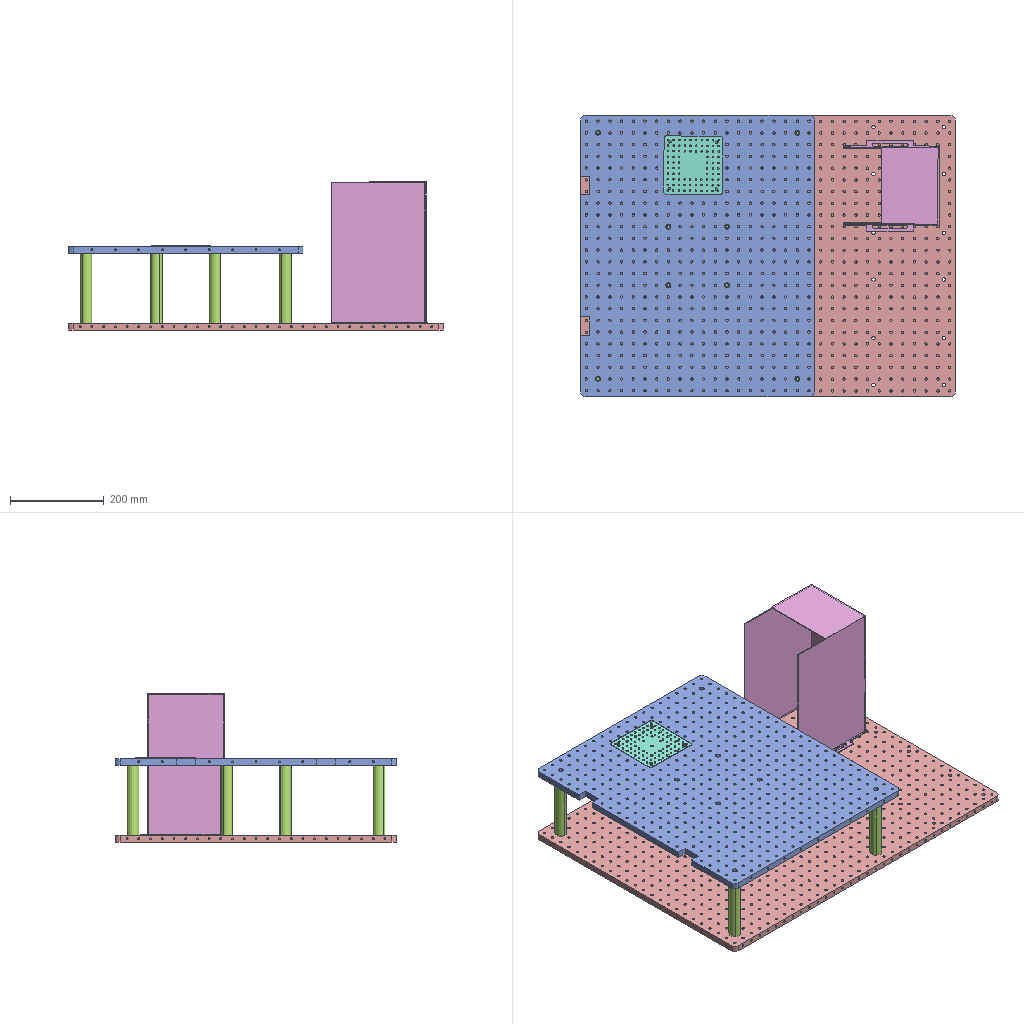Assembly | SolidWorks | 5 different items | 12 placed | box 800 x 600 x 316 mm
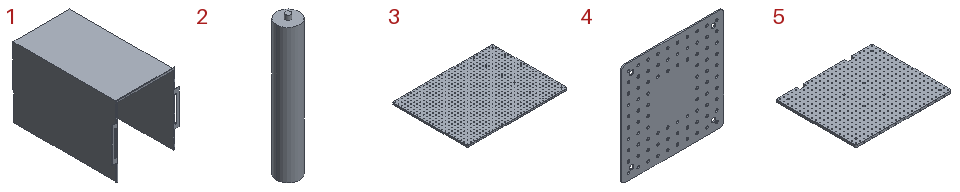Parts list (item | quantity | size | volume | features):
1 | x1 | 194 x 302 x 205 mm | 384147 mm3 | features ICE 4, Extrusion 1
2 | x8 | 25.4 x 25.4 x 155 mm | 75865 mm3 | features BaseBody 1
3 | x1 | 800 x 600 x 14 mm | 6524113 mm3 | features BaseBody 1
4 | x1 | 125 x 1.5 x 125 mm | 22249 mm3 | features ICE 3, BaseBody 1
5 | x1 | 600 x 500 x 14 mm | 4024058 mm3 | features BaseBody 1
Mates (type | each side: item.copy, entity, surface, feature):
Coincident | 3.1 face plane Input1 | 1.1 face plane Boss-Extrude1
Coincident | 5.1 face plane Input1 | 4.1 face plane Cut-Extrude3